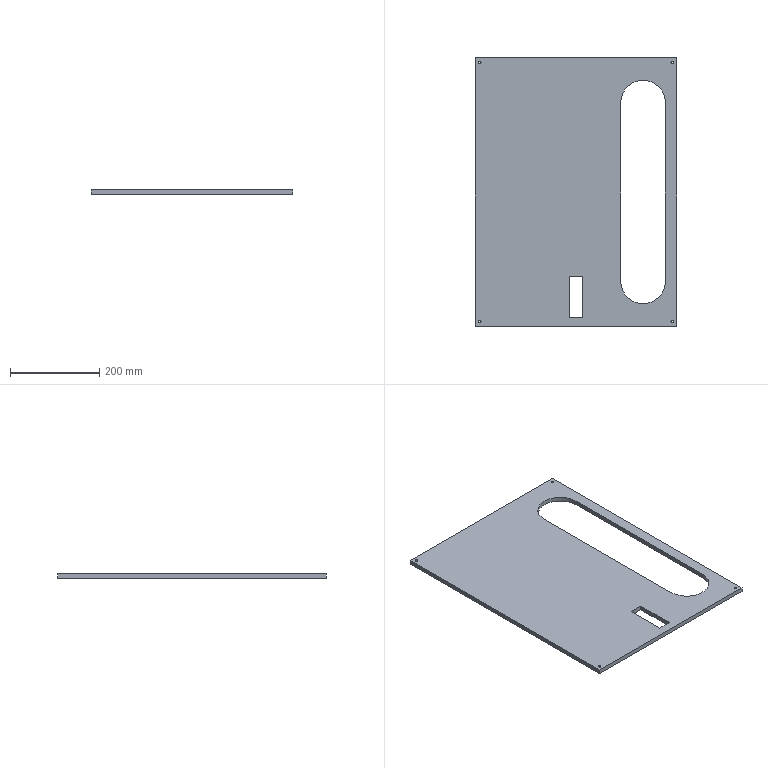Part | STEP file | B1-024 | 1 solid | 22 faces | box 450 x 600 x 10 mm | volume 2193510 mm3 | plane 12 | cylinder 10 | commonest cylinder face diameters 5.5 x8 100 x2